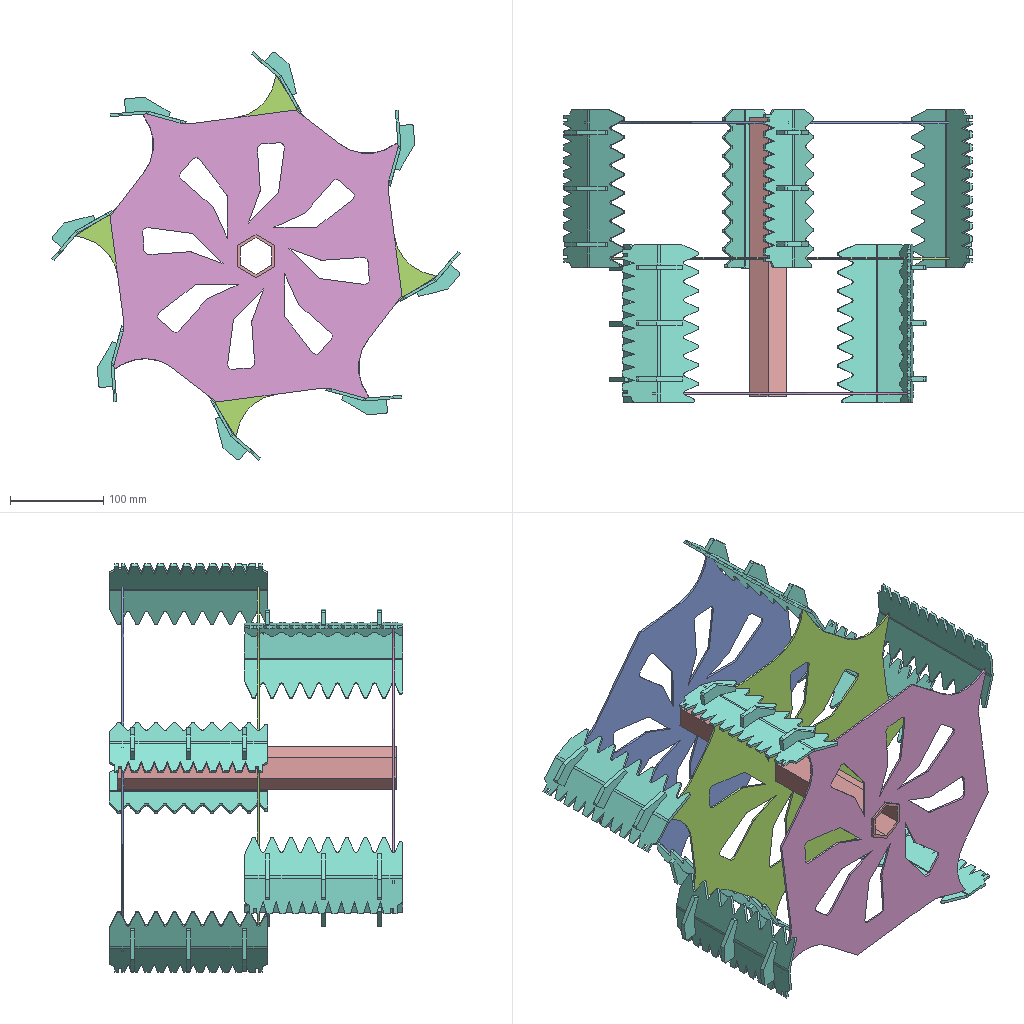Assembly | SolidWorks | 5 different items | 12 placed | box 438 x 315 x 438 mm
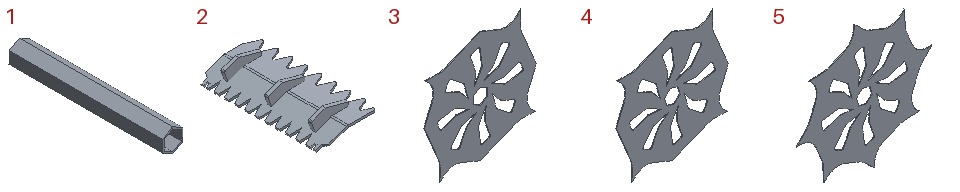Parts list (item | quantity | size | volume | features):
1 | x1 | 40 x 300 x 46.188 mm | 115355 mm3 | features Extrusion 1
2 | x8 | 81.389 x 170 x 29.968 mm | 44685 mm3 | features BaseBody 1, ICE 1, MirrorSolid 1
3 | x1 | 324.718 x 2 x 324.718 mm | 127510 mm3 | features ICE 3, Extrusion 1, Fillet 1
4 | x1 | 324.718 x 2 x 324.718 mm | 127510 mm3 | features ICE 3, Extrusion 1, Fillet 1
5 | x1 | 387.128 x 2 x 387.128 mm | 134458 mm3 | features ICE 3, Extrusion 1, Fillet 1
Mates (type | each side: item.copy, entity, surface, feature):
Coincident | 1.1 face plane Boss-Extrude1 | 3.1 face plane Cut-Extrude1 | 2 times
DistanceDim | 1.1 face plane Boss-Extrude1 | 3.1 face plane Boss-Extrude1
Coincident | 3.1 face plane Boss-Extrude1 | 5.1 face plane Boss-Extrude1 | 2 times
Coincident | 5.1 face plane Boss-Extrude1 | 4.1 face plane Boss-Extrude1
Coincident | 1.1 face plane Boss-Extrude1 | 4.1 face plane Cut-Extrude1
DistanceDim | 4.1 face plane Boss-Extrude1 | 1.1 face plane Boss-Extrude1
Width | 5.1 face plane Boss-Extrude1 | 5.1 face plane Boss-Extrude1 | 3.1 face plane Boss-Extrude1 | 4.1 face plane Boss-Extrude1
Coincident | 1.1 plane | assembly plane | 2 times
Coincident | 3.1 face plane Boss-Extrude2 | 2.1 face plane Mirror6
Parallel | 3.1 face plane Boss-Extrude1 | 2.1 face plane Mirror6
Parallel | 4.1 face plane Boss-Extrude1 | 2.2 face plane Mirror6
Coincident | 4.1 face plane Boss-Extrude2 | 2.2 face plane Mirror6